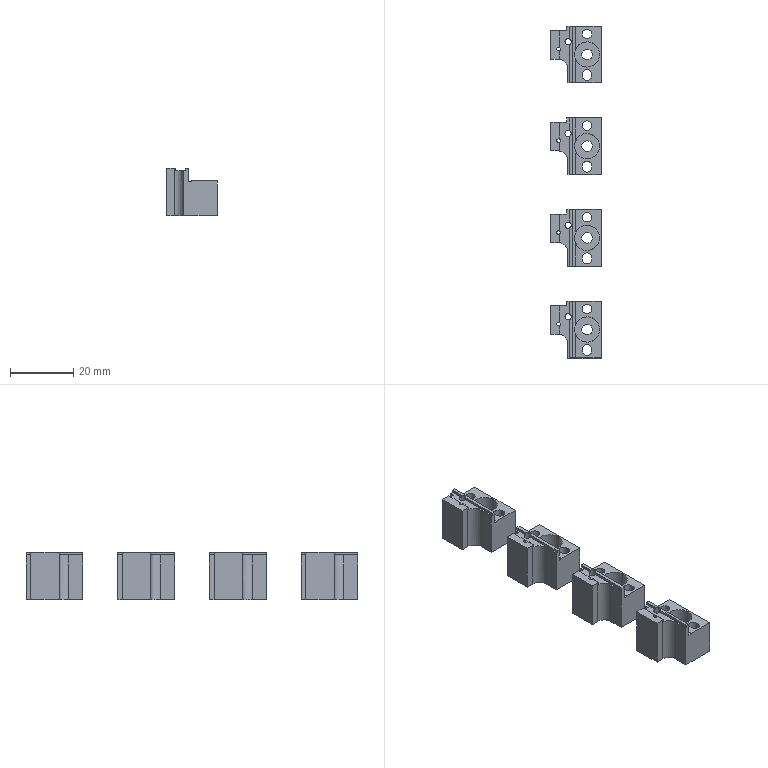CAM job | NX | 3-axis milling, drilling | part box 16 x 105 x 15 mm | stock box 20 x 110 x 20 mm
Tools:
number,name,description,diameter,corner_radius,flute_length,length,flutes
20,D2,平底铣刀-粗,2.0,0.0,50.0,75.0,2
4,D4,平底铣刀-粗,4.0,0.0,25.0,75.0,2
9,D10,平底铣刀-粗,10.0,0.0,35.0,75.0,2
22,D2-J,平底铣刀-精,2.0,0.0,50.0,75.0,2
11,D4-J,平底铣刀-精,4.0,0.0,50.0,75.0,2
7,D6-J,平底铣刀-精,6.0,0.0,25.0,75.0,2
10,D10-J,平底铣刀-精,10.0,0.0,35.0,75.0,2
2,D6倒角刀,倒角刀,6.0,0.0,3.0,25.0,2
17,ZT1.2,钻头,1.2,0.0,35.0,50.0,2
13,ZT3.4,钻头,3.4,0.0,35.0,50.0,2
19,ZT2.9,Drilling Tool,2.9,0.0,35.0,50.0,2
18,ZT1.9,Drilling Tool,1.9,0.0,35.0,50.0,2
23,D2REAMER,Drilling Tool,1.95,0.0,20.0,50.0,4
Operations:
program,operation,operation_type,tool,method,geometry_group,spindle_rpm,surface_speed,feed_per_tooth,feed_cut,feed_plunge,cut_length_mm,path_length_mm,cut_time_min,machine_time_min
A,顶面,FaceMilling,D10-J,侧刃精光-切深K-步距G,W-A,8000.0,251.327,0.0625,1000.0,100.0,372.0,408.0,0.372,0.3756
A,外形粗_2,VolumeBased25DMillingOperation,D10,METHOD,W-A,8000.0,251.327,0.3125,5000.0,80.0,8133.852,8433.352,1.627,1.657
A,打点-深0.8,Operation,D6倒角刀,NONE,W-A,8000.0,150.796,0.0312,500.0,90.0,36.0,373.823,0.072,0.1058
A,通孔-1-2,Operation,ZT1.2,NONE,W-A,3000.0,11.31,0.0033,20.0,90.0,17.442,164.936,0.8721,0.8869
A,通孔-1-2_2,Operation,ZT1.9,NONE,W-A,3000.0,18.85,0.005,30.0,90.0,84.0,298.052,2.8,2.821
A,通孔-精孔3.0预钻,Operation,ZT2.9,NONE,W-A,3200.0,29.154,0.0312,200.0,90.0,158.697,638.253,0.7935,0.8414
A,沉头孔-钻孔0段,Operation,ZT3.4,NONE,W-A,2800.0,29.908,0.0357,200.0,90.0,76.086,282.223,0.3804,0.401
A,底壁铣分层开粗-中_COPY,VolumeBased25DMillingOperation,D10,分层开粗-切深K-步距G,W-A,8000.0,251.32,0.25,4000.0,100.0,1556.5,1582.443,0.3891,0.3917
A,通腰槽粗_1,VolumeBased25DMillingOperation,D2,METHOD,W-A,6000.0,37.699,0.05,600.0,100.0,1650.861,1966.409,2.751,2.783
A,底壁铣分层开粗-中_COPY_1,VolumeBased25DMillingOperation,D2,分层开粗-切深K-步距G,W-A,8000.0,100.528,0.125,2000.0,100.0,1469.833,1643.37,0.7349,0.7523
A,铣孔开粗D4_1,CylinderMilling,D4,NONE,W-A,8000.0,100.531,0.075,1200.0,100.0,1106.586,1436.586,0.9222,0.9552
A,铣孔精光D4_1,CylinderMilling,D4-J,精光步距切深关,W-A,8000.0,100.531,0.0312,500.0,100.0,145.496,475.496,0.291,0.324
A,外形侧面,ZLevelMilling,D2-J,METHOD,W-A,9000.0,56.549,0.1111,2000.0,80.0,8185.539,9271.945,4.096,4.205
A,底壁铣精光底面-中_COPY,VolumeBased25DMillingOperation,D6-J,精光步距切深关,W-A,7000.0,175.0,0.0536,1500.0,100.0,578.046,749.33,0.3854,0.4025
A,仅选体,SurfaceContour,D6倒角刀,METHOD,W-A,8000.0,150.796,0.1875,3000.0,100.0,651.465,1252.707,0.2172,0.2773
A,钻倒角_1,Operation,D6倒角刀,METHOD,W-A,8000.0,150.796,0.0312,500.0,0.0,15.6,167.664,0.0312,0.0464
A,钻倒角_2,Operation,D6倒角刀,METHOD,W-A,8000.0,150.796,0.0312,500.0,0.0,17.2,170.864,0.0344,0.0498
A,钻倒角_3,Operation,D6倒角刀,METHOD,W-A,8000.0,150.796,0.0312,500.0,0.0,19.2,182.864,0.0384,0.0548
A,底壁铣精光侧面-中-选底面_COPY,VolumeBased25DMillingOperation,D2-J,侧刃精光-切深K-步距G,W-A,8000.0,100.528,0.05,800.0,100.0,151.086,253.519,0.1889,0.1991
A,腰槽精_1,VolumeBased25DMillingOperation,D2-J,METHOD,W-A,6000.0,113.0,0.0167,200.0,100.0,290.038,1126.567,1.45,1.534
A,REAMING_COPY,Operation,D2REAMER,METHOD,W-A,500.0,4.712,0.0167,50.0,0.0,68.0,266.052,1.36,1.38
A,外形半精_2,VolumeBased25DMillingOperation,D6-J,METHOD,W-A,8000.0,251.327,0.0625,1000.0,100.0,358.087,728.639,0.3581,0.3951
A,等高精光-中_COPY,ZLevelMilling,D6-J,侧刃精光-切深K-步距G,W-A,8000.0,150.792,0.0625,1000.0,100.0,114.594,327.546,0.1146,0.1359